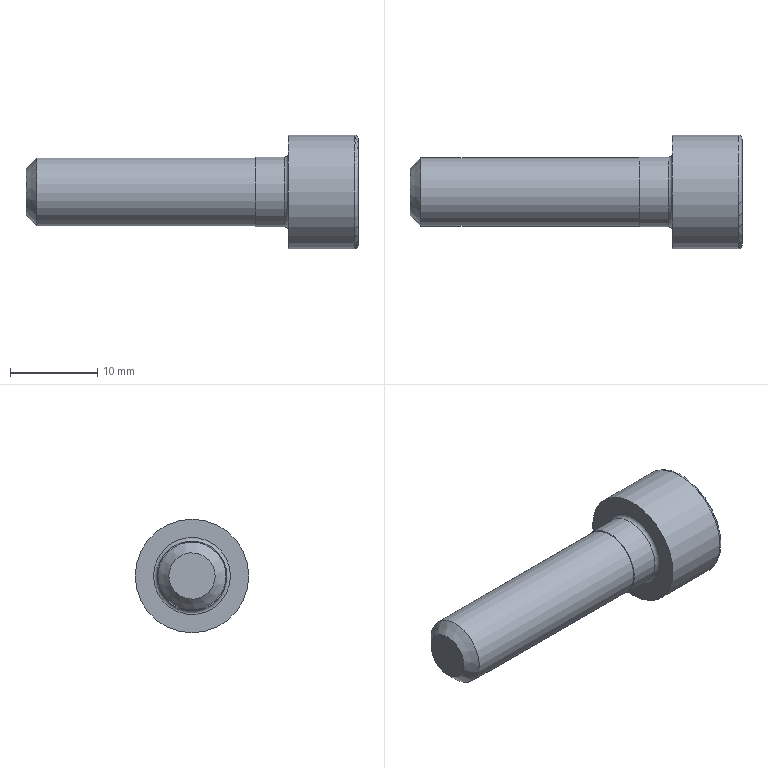Part | STEP file | PARAFUSO_DIN 912_M8x30 | 1 solid | 24 faces | box 38 x 13 x 13 mm | volume 2340 mm3 | plane 11 | cylinder 9 | torus 2 | cone 2 | commonest cylinder face diameters 6.863 x6 7.805 x1 8 x1 13 x1